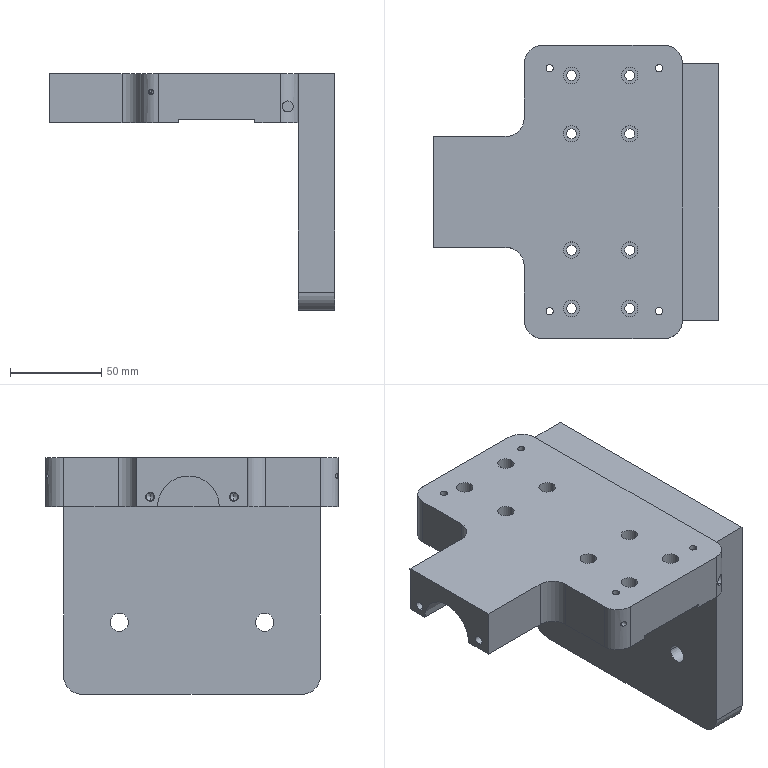Part | SolidWorks | features ICE 9, Fillet 2, BaseBody 1, MoveFace 1 | 2 solids | 164 faces | box 156.892 x 161 x 130 mm | volume 769090 mm3 | cylinder 105 | plane 43 | cone 16 | commonest cylinder face diameters 5.5 x16 6 x16 9 x16 5 x14 4.2 x10 4 x8